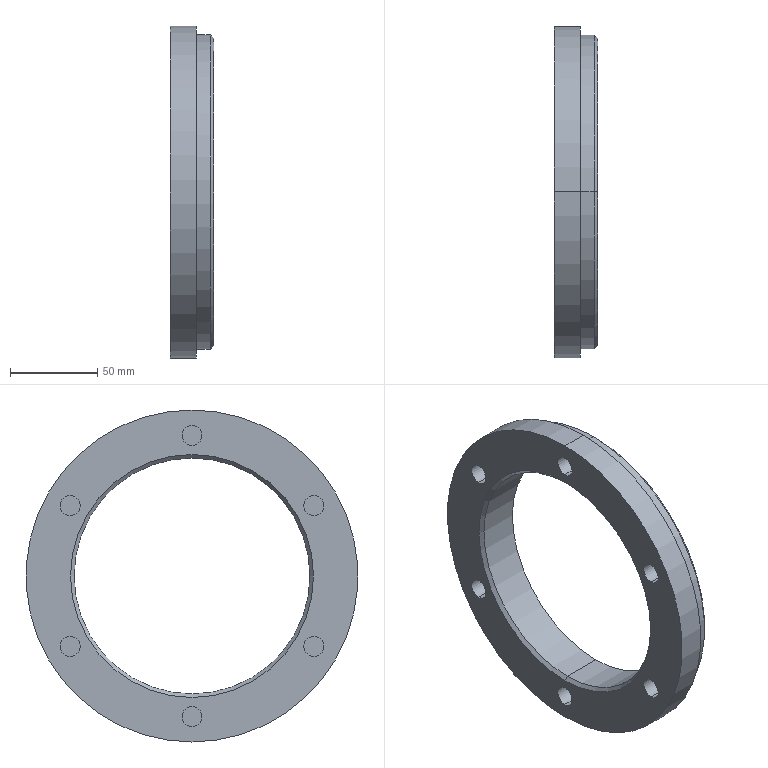Part | SolidWorks | features ICE 2, Chamfer 1, Extrusion 1 | 1 solid | 31 faces | box 25 x 190 x 190 mm | volume 309030 mm3 | cylinder 18 | plane 9 | cone 4 | commonest cylinder face diameters 11.5 x12 135 x2 180 x2 190 x2
STEP:
#1=CARTESIAN_POINT('',(25.,0.,-88.));
#2=VERTEX_POINT('',#1);
#3=CARTESIAN_POINT('',(25.,0.,88.));
#4=VERTEX_POINT('',#3);
#5=CARTESIAN_POINT('',(25.,0.,0.));
#6=DIRECTION('',(1.,0.,0.));
#7=DIRECTION('',(0.,0.,-1.));
#8=AXIS2_PLACEMENT_3D('',#5,#6,#7);
#9=CIRCLE('',#8,88.);
#10=EDGE_CURVE('',#2,#4,#9,.T.);
#11=ORIENTED_EDGE('',*,*,#10,.F.);
#12=CARTESIAN_POINT('',(23.,0.,-90.));
#13=VERTEX_POINT('',#12);
#14=CARTESIAN_POINT('',(25.,0.,-88.));
#15=DIRECTION('',(-0.7071,0.,-0.7071));
#16=VECTOR('',#15,1000.);
#17=LINE('',#14,#16);
#18=EDGE_CURVE('',#2,#13,#17,.T.);
#19=ORIENTED_EDGE('',*,*,#18,.T.);
#20=CARTESIAN_POINT('',(23.,0.,90.));
#21=VERTEX_POINT('',#20);
#22=CARTESIAN_POINT('',(23.,0.,0.));
#23=DIRECTION('',(-1.,0.,0.));
#24=DIRECTION('',(0.,0.,-1.));
#25=AXIS2_PLACEMENT_3D('',#22,#23,#24);
#26=CIRCLE('',#25,90.);
#27=EDGE_CURVE('',#21,#13,#26,.T.);
#28=ORIENTED_EDGE('',*,*,#27,.F.);
#29=CARTESIAN_POINT('',(25.,0.,88.));
#30=DIRECTION('',(-0.7071,0.,0.7071));
#31=VECTOR('',#30,1000.);
#32=LINE('',#29,#31);
#33=EDGE_CURVE('',#4,#21,#32,.T.);
#34=ORIENTED_EDGE('',*,*,#33,.F.);
#35=EDGE_LOOP('',(#11,#19,#28,#34));
#36=FACE_OUTER_BOUND('',#35,.T.);
#37=CARTESIAN_POINT('',(25.,0.,0.));
#38=DIRECTION('',(-1.,0.,0.));
#39=DIRECTION('',(0.,0.,1.));
#40=AXIS2_PLACEMENT_3D('',#37,#38,#39);
#41=CONICAL_SURFACE('',#40,88.,0.7854);
#42=ADVANCED_FACE('',(#36),#41,.T.);
#43=CARTESIAN_POINT('',(2.,0.,-67.5));
#44=VERTEX_POINT('',#43);
#45=CARTESIAN_POINT('',(2.,0.,67.5));
#46=VERTEX_POINT('',#45);
#47=CARTESIAN_POINT('',(2.,0.,0.));
#48=DIRECTION('',(-1.,0.,0.));
#49=DIRECTION('',(0.,0.,-1.));
#50=AXIS2_PLACEMENT_3D('',#47,#48,#49);
#51=CIRCLE('',#50,67.5);
#52=EDGE_CURVE('',#44,#46,#51,.T.);
#53=ORIENTED_EDGE('',*,*,#52,.F.);
#54=CARTESIAN_POINT('',(0.,0.,-69.5));
#55=VERTEX_POINT('',#54);
#56=CARTESIAN_POINT('',(0.,0.,-69.5));
#57=DIRECTION('',(-0.7071,0.,-0.7071));
#58=VECTOR('',#57,1000.);
#59=LINE('',#56,#58);
#60=EDGE_CURVE('',#44,#55,#59,.T.);
#61=ORIENTED_EDGE('',*,*,#60,.T.);
#62=CARTESIAN_POINT('',(0.,0.,69.5));
#63=VERTEX_POINT('',#62);
#64=CARTESIAN_POINT('',(0.,0.,0.));
#65=DIRECTION('',(1.,0.,0.));
#66=DIRECTION('',(0.,0.,-1.));
#67=AXIS2_PLACEMENT_3D('',#64,#65,#66);
#68=CIRCLE('',#67,69.5);
#69=EDGE_CURVE('',#63,#55,#68,.T.);
#70=ORIENTED_EDGE('',*,*,#69,.F.);
#71=CARTESIAN_POINT('',(0.,0.,69.5));
#72=DIRECTION('',(-0.7071,0.,0.7071));
#73=VECTOR('',#72,1000.);
#74=LINE('',#71,#73);
#75=EDGE_CURVE('',#46,#63,#74,.T.);
#76=ORIENTED_EDGE('',*,*,#75,.F.);
#77=EDGE_LOOP('',(#53,#61,#70,#76));
#78=FACE_OUTER_BOUND('',#77,.T.);
#79=CARTESIAN_POINT('',(0.,0.,0.));
#80=DIRECTION('',(-1.,0.,0.));
#81=DIRECTION('',(0.,0.,1.));
#82=AXIS2_PLACEMENT_3D('',#79,#80,#81);
#83=CONICAL_SURFACE('',#82,69.5,0.7854);
#84=ADVANCED_FACE('',(#78),#83,.F.);
#85=CARTESIAN_POINT('',(17.5,69.715,34.5));
#86=VERTEX_POINT('',#85);
#87=CARTESIAN_POINT('',(17.5,69.715,46.));
#88=VERTEX_POINT('',#87);
#89=CARTESIAN_POINT('',(17.5,69.715,40.25));
#90=DIRECTION('',(-1.,0.,0.));
#91=DIRECTION('',(0.,0.,1.));
#92=AXIS2_PLACEMENT_3D('',#89,#90,#91);
#93=CIRCLE('',#92,5.75);
#94=EDGE_CURVE('',#86,#88,#93,.T.);
#95=ORIENTED_EDGE('',*,*,#94,.F.);
#96=CARTESIAN_POINT('',(0.,69.715,34.5));
#97=VERTEX_POINT('',#96);
#98=CARTESIAN_POINT('',(17.5,69.715,34.5));
#99=DIRECTION('',(-1.,0.,0.));
#100=VECTOR('',#99,1000.);
#101=LINE('',#98,#100);
#102=EDGE_CURVE('',#86,#97,#101,.T.);
#103=ORIENTED_EDGE('',*,*,#102,.T.);
#104=CARTESIAN_POINT('',(0.,69.715,46.));
#105=VERTEX_POINT('',#104);
#106=CARTESIAN_POINT('',(0.,69.715,40.25));
#107=DIRECTION('',(-1.,0.,0.));
#108=DIRECTION('',(0.,0.,1.));
#109=AXIS2_PLACEMENT_3D('',#106,#107,#108);
#110=CIRCLE('',#109,5.75);
#111=EDGE_CURVE('',#97,#105,#110,.T.);
#112=ORIENTED_EDGE('',*,*,#111,.T.);
#113=CARTESIAN_POINT('',(17.5,69.715,46.));
#114=DIRECTION('',(-1.,0.,0.));
#115=VECTOR('',#114,1000.);
#116=LINE('',#113,#115);
#117=EDGE_CURVE('',#88,#105,#116,.T.);
#118=ORIENTED_EDGE('',*,*,#117,.F.);
#119=EDGE_LOOP('',(#95,#103,#112,#118));
#120=FACE_OUTER_BOUND('',#119,.T.);
#121=CARTESIAN_POINT('',(17.5,69.715,40.25));
#122=DIRECTION('',(-1.,0.,0.));
#123=DIRECTION('',(0.,0.,1.));
#124=AXIS2_PLACEMENT_3D('',#121,#122,#123);
#125=CYLINDRICAL_SURFACE('',#124,5.75);
#126=ADVANCED_FACE('',(#120),#125,.F.);
#127=CARTESIAN_POINT('',(17.5,69.715,-46.));
#128=VERTEX_POINT('',#127);
#129=CARTESIAN_POINT('',(17.5,69.715,-34.5));
#130=VERTEX_POINT('',#129);
#131=CARTESIAN_POINT('',(17.5,69.715,-40.25));
#132=DIRECTION('',(-1.,0.,0.));
#133=DIRECTION('',(0.,0.,1.));
#134=AXIS2_PLACEMENT_3D('',#131,#132,#133);
#135=CIRCLE('',#134,5.75);
#136=EDGE_CURVE('',#128,#130,#135,.T.);
#137=ORIENTED_EDGE('',*,*,#136,.F.);
#138=CARTESIAN_POINT('',(0.,69.715,-46.));
#139=VERTEX_POINT('',#138);
#140=CARTESIAN_POINT('',(17.5,69.715,-46.));
#141=DIRECTION('',(-1.,0.,0.));
#142=VECTOR('',#141,1000.);
#143=LINE('',#140,#142);
#144=EDGE_CURVE('',#128,#139,#143,.T.);
#145=ORIENTED_EDGE('',*,*,#144,.T.);
#146=CARTESIAN_POINT('',(0.,69.715,-34.5));
#147=VERTEX_POINT('',#146);
#148=CARTESIAN_POINT('',(0.,69.715,-40.25));
#149=DIRECTION('',(-1.,0.,0.));
#150=DIRECTION('',(0.,0.,1.));
#151=AXIS2_PLACEMENT_3D('',#148,#149,#150);
#152=CIRCLE('',#151,5.75);
#153=EDGE_CURVE('',#139,#147,#152,.T.);
#154=ORIENTED_EDGE('',*,*,#153,.T.);
#155=CARTESIAN_POINT('',(17.5,69.715,-34.5));
#156=DIRECTION('',(-1.,0.,0.));
#157=VECTOR('',#156,1000.);
#158=LINE('',#155,#157);
#159=EDGE_CURVE('',#130,#147,#158,.T.);
#160=ORIENTED_EDGE('',*,*,#159,.F.);
#161=EDGE_LOOP('',(#137,#145,#154,#160));
#162=FACE_OUTER_BOUND('',#161,.T.);
#163=CARTESIAN_POINT('',(17.5,69.715,-40.25));
#164=DIRECTION('',(-1.,0.,0.));
#165=DIRECTION('',(0.,0.,1.));
#166=AXIS2_PLACEMENT_3D('',#163,#164,#165);
#167=CYLINDRICAL_SURFACE('',#166,5.75);
#168=ADVANCED_FACE('',(#162),#167,.F.);
#169=CARTESIAN_POINT('',(17.5,0.,-86.25));
#170=VERTEX_POINT('',#169);
#171=CARTESIAN_POINT('',(17.5,0.,-74.75));
#172=VERTEX_POINT('',#171);
#173=CARTESIAN_POINT('',(17.5,0.,-80.5));
#174=DIRECTION('',(-1.,0.,0.));
#175=DIRECTION('',(0.,0.,1.));
#176=AXIS2_PLACEMENT_3D('',#173,#174,#175);
#177=CIRCLE('',#176,5.75);
#178=EDGE_CURVE('',#170,#172,#177,.T.);
#179=ORIENTED_EDGE('',*,*,#178,.F.);
#180=CARTESIAN_POINT('',(0.,0.,-86.25));
#181=VERTEX_POINT('',#180);
#182=CARTESIAN_POINT('',(17.5,0.,-86.25));
#183=DIRECTION('',(-1.,0.,0.));
#184=VECTOR('',#183,1000.);
#185=LINE('',#182,#184);
#186=EDGE_CURVE('',#170,#181,#185,.T.);
#187=ORIENTED_EDGE('',*,*,#186,.T.);
#188=CARTESIAN_POINT('',(0.,0.,-74.75));
#189=VERTEX_POINT('',#188);
#190=CARTESIAN_POINT('',(0.,0.,-80.5));
#191=DIRECTION('',(-1.,0.,0.));
#192=DIRECTION('',(0.,0.,1.));
#193=AXIS2_PLACEMENT_3D('',#190,#191,#192);
#194=CIRCLE('',#193,5.75);
#195=EDGE_CURVE('',#181,#189,#194,.T.);
#196=ORIENTED_EDGE('',*,*,#195,.T.);
#197=CARTESIAN_POINT('',(17.5,0.,-74.75));
#198=DIRECTION('',(-1.,0.,0.));
#199=VECTOR('',#198,1000.);
#200=LINE('',#197,#199);
#201=EDGE_CURVE('',#172,#189,#200,.T.);
#202=ORIENTED_EDGE('',*,*,#201,.F.);
#203=EDGE_LOOP('',(#179,#187,#196,#202));
#204=FACE_OUTER_BOUND('',#203,.T.);
#205=CARTESIAN_POINT('',(17.5,0.,-80.5));
#206=DIRECTION('',(-1.,0.,0.));
#207=DIRECTION('',(0.,0.,1.));
#208=AXIS2_PLACEMENT_3D('',#205,#206,#207);
#209=CYLINDRICAL_SURFACE('',#208,5.75);
#210=ADVANCED_FACE('',(#204),#209,.F.);
#211=CARTESIAN_POINT('',(17.5,-69.715,-46.));
#212=VERTEX_POINT('',#211);
#213=CARTESIAN_POINT('',(17.5,-69.715,-34.5));
#214=VERTEX_POINT('',#213);
#215=CARTESIAN_POINT('',(17.5,-69.715,-40.25));
#216=DIRECTION('',(-1.,0.,0.));
#217=DIRECTION('',(0.,0.,1.));
#218=AXIS2_PLACEMENT_3D('',#215,#216,#217);
#219=CIRCLE('',#218,5.75);
#220=EDGE_CURVE('',#212,#214,#219,.T.);
#221=ORIENTED_EDGE('',*,*,#220,.F.);
#222=CARTESIAN_POINT('',(0.,-69.715,-46.));
#223=VERTEX_POINT('',#222);
#224=CARTESIAN_POINT('',(17.5,-69.715,-46.));
#225=DIRECTION('',(-1.,0.,0.));
#226=VECTOR('',#225,1000.);
#227=LINE('',#224,#226);
#228=EDGE_CURVE('',#212,#223,#227,.T.);
#229=ORIENTED_EDGE('',*,*,#228,.T.);
#230=CARTESIAN_POINT('',(0.,-69.715,-34.5));
#231=VERTEX_POINT('',#230);
#232=CARTESIAN_POINT('',(0.,-69.715,-40.25));
#233=DIRECTION('',(-1.,0.,0.));
#234=DIRECTION('',(0.,0.,1.));
#235=AXIS2_PLACEMENT_3D('',#232,#233,#234);
#236=CIRCLE('',#235,5.75);
#237=EDGE_CURVE('',#223,#231,#236,.T.);
#238=ORIENTED_EDGE('',*,*,#237,.T.);
#239=CARTESIAN_POINT('',(17.5,-69.715,-34.5));
#240=DIRECTION('',(-1.,0.,0.));
#241=VECTOR('',#240,1000.);
#242=LINE('',#239,#241);
#243=EDGE_CURVE('',#214,#231,#242,.T.);
#244=ORIENTED_EDGE('',*,*,#243,.F.);
#245=EDGE_LOOP('',(#221,#229,#238,#244));
#246=FACE_OUTER_BOUND('',#245,.T.);
#247=CARTESIAN_POINT('',(17.5,-69.715,-40.25));
#248=DIRECTION('',(-1.,0.,0.));
#249=DIRECTION('',(0.,0.,1.));
#250=AXIS2_PLACEMENT_3D('',#247,#248,#249);
#251=CYLINDRICAL_SURFACE('',#250,5.75);
#252=ADVANCED_FACE('',(#246),#251,.F.);
#253=CARTESIAN_POINT('',(17.5,-69.715,34.5));
#254=VERTEX_POINT('',#253);
#255=CARTESIAN_POINT('',(17.5,-69.715,46.));
#256=VERTEX_POINT('',#255);
#257=CARTESIAN_POINT('',(17.5,-69.715,40.25));
#258=DIRECTION('',(-1.,0.,0.));
#259=DIRECTION('',(0.,0.,1.));
#260=AXIS2_PLACEMENT_3D('',#257,#258,#259);
#261=CIRCLE('',#260,5.75);
#262=EDGE_CURVE('',#254,#256,#261,.T.);
#263=ORIENTED_EDGE('',*,*,#262,.F.);
#264=CARTESIAN_POINT('',(0.,-69.715,34.5));
#265=VERTEX_POINT('',#264);
#266=CARTESIAN_POINT('',(17.5,-69.715,34.5));
#267=DIRECTION('',(-1.,0.,0.));
#268=VECTOR('',#267,1000.);
#269=LINE('',#266,#268);
#270=EDGE_CURVE('',#254,#265,#269,.T.);
#271=ORIENTED_EDGE('',*,*,#270,.T.);
#272=CARTESIAN_POINT('',(0.,-69.715,46.));
#273=VERTEX_POINT('',#272);
#274=CARTESIAN_POINT('',(0.,-69.715,40.25));
#275=DIRECTION('',(-1.,0.,0.));
#276=DIRECTION('',(0.,0.,1.));
#277=AXIS2_PLACEMENT_3D('',#274,#275,#276);
#278=CIRCLE('',#277,5.75);
#279=EDGE_CURVE('',#265,#273,#278,.T.);
#280=ORIENTED_EDGE('',*,*,#279,.T.);
#281=CARTESIAN_POINT('',(17.5,-69.715,46.));
#282=DIRECTION('',(-1.,0.,0.));
#283=VECTOR('',#282,1000.);
#284=LINE('',#281,#283);
#285=EDGE_CURVE('',#256,#273,#284,.T.);
#286=ORIENTED_EDGE('',*,*,#285,.F.);
#287=EDGE_LOOP('',(#263,#271,#280,#286));
#288=FACE_OUTER_BOUND('',#287,.T.);
#289=CARTESIAN_POINT('',(17.5,-69.715,40.25));
#290=DIRECTION('',(-1.,0.,0.));
#291=DIRECTION('',(0.,0.,1.));
#292=AXIS2_PLACEMENT_3D('',#289,#290,#291);
#293=CYLINDRICAL_SURFACE('',#292,5.75);
#294=ADVANCED_FACE('',(#288),#293,.F.);
#295=CARTESIAN_POINT('',(17.5,0.,74.75));
#296=VERTEX_POINT('',#295);
#297=CARTESIAN_POINT('',(17.5,0.,86.25));
#298=VERTEX_POINT('',#297);
#299=CARTESIAN_POINT('',(17.5,0.,80.5));
#300=DIRECTION('',(-1.,0.,0.));
#301=DIRECTION('',(0.,0.,1.));
#302=AXIS2_PLACEMENT_3D('',#299,#300,#301);
#303=CIRCLE('',#302,5.75);
#304=EDGE_CURVE('',#296,#298,#303,.T.);
#305=ORIENTED_EDGE('',*,*,#304,.F.);
#306=CARTESIAN_POINT('',(0.,0.,74.75));
#307=VERTEX_POINT('',#306);
#308=CARTESIAN_POINT('',(17.5,0.,74.75));
#309=DIRECTION('',(-1.,0.,0.));
#310=VECTOR('',#309,1000.);
#311=LINE('',#308,#310);
#312=EDGE_CURVE('',#296,#307,#311,.T.);
#313=ORIENTED_EDGE('',*,*,#312,.T.);
#314=CARTESIAN_POINT('',(0.,0.,86.25));
#315=VERTEX_POINT('',#314);
#316=CARTESIAN_POINT('',(0.,0.,80.5));
#317=DIRECTION('',(-1.,0.,0.));
#318=DIRECTION('',(0.,0.,1.));
#319=AXIS2_PLACEMENT_3D('',#316,#317,#318);
#320=CIRCLE('',#319,5.75);
#321=EDGE_CURVE('',#307,#315,#320,.T.);
#322=ORIENTED_EDGE('',*,*,#321,.T.);
#323=CARTESIAN_POINT('',(17.5,0.,86.25));
#324=DIRECTION('',(-1.,0.,0.));
#325=VECTOR('',#324,1000.);
#326=LINE('',#323,#325);
#327=EDGE_CURVE('',#298,#315,#326,.T.);
#328=ORIENTED_EDGE('',*,*,#327,.F.);
#329=EDGE_LOOP('',(#305,#313,#322,#328));
#330=FACE_OUTER_BOUND('',#329,.T.);
#331=CARTESIAN_POINT('',(17.5,0.,80.5));
#332=DIRECTION('',(-1.,0.,0.));
#333=DIRECTION('',(0.,0.,1.));
#334=AXIS2_PLACEMENT_3D('',#331,#332,#333);
#335=CYLINDRICAL_SURFACE('',#334,5.75);
#336=ADVANCED_FACE('',(#330),#335,.F.);
#337=CARTESIAN_POINT('',(15.,0.,-90.));
#338=VERTEX_POINT('',#337);
#339=CARTESIAN_POINT('',(15.,0.,90.));
#340=VERTEX_POINT('',#339);
#341=CARTESIAN_POINT('',(15.,0.,0.));
#342=DIRECTION('',(1.,0.,0.));
#343=DIRECTION('',(0.,0.,-1.));
#344=AXIS2_PLACEMENT_3D('',#341,#342,#343);
#345=CIRCLE('',#344,90.);
#346=EDGE_CURVE('',#338,#340,#345,.T.);
#347=ORIENTED_EDGE('',*,*,#346,.T.);
#348=CARTESIAN_POINT('',(15.,0.,90.));
#349=DIRECTION('',(1.,0.,0.));
#350=VECTOR('',#349,1000.);
#351=LINE('',#348,#350);
#352=EDGE_CURVE('',#340,#21,#351,.T.);
#353=ORIENTED_EDGE('',*,*,#352,.T.);
#354=ORIENTED_EDGE('',*,*,#27,.T.);
#355=CARTESIAN_POINT('',(15.,0.,-90.));
#356=DIRECTION('',(1.,0.,0.));
#357=VECTOR('',#356,1000.);
#358=LINE('',#355,#357);
#359=EDGE_CURVE('',#338,#13,#358,.T.);
#360=ORIENTED_EDGE('',*,*,#359,.F.);
#361=EDGE_LOOP('',(#347,#353,#354,#360));
#362=FACE_OUTER_BOUND('',#361,.T.);
#363=CARTESIAN_POINT('',(15.,0.,0.));
#364=DIRECTION('',(1.,0.,0.));
#365=DIRECTION('',(0.,0.,-1.));
#366=AXIS2_PLACEMENT_3D('',#363,#364,#365);
#367=CYLINDRICAL_SURFACE('',#366,90.);
#368=ADVANCED_FACE('',(#362),#367,.T.);
#369=CARTESIAN_POINT('',(25.,0.,67.5));
#370=VERTEX_POINT('',#369);
#371=CARTESIAN_POINT('',(25.,0.,-67.5));
#372=VERTEX_POINT('',#371);
#373=CARTESIAN_POINT('',(25.,0.,0.));
#374=DIRECTION('',(1.,0.,0.));
#375=DIRECTION('',(0.,0.,-1.));
#376=AXIS2_PLACEMENT_3D('',#373,#374,#375);
#377=CIRCLE('',#376,67.5);
#378=EDGE_CURVE('',#370,#372,#377,.T.);
#379=ORIENTED_EDGE('',*,*,#378,.T.);
#380=CARTESIAN_POINT('',(25.,0.,-67.5));
#381=DIRECTION('',(-1.,0.,0.));
#382=VECTOR('',#381,1000.);
#383=LINE('',#380,#382);
#384=EDGE_CURVE('',#372,#44,#383,.T.);
#385=ORIENTED_EDGE('',*,*,#384,.T.);
#386=ORIENTED_EDGE('',*,*,#52,.T.);
#387=CARTESIAN_POINT('',(25.,0.,67.5));
#388=DIRECTION('',(-1.,0.,0.));
#389=VECTOR('',#388,1000.);
#390=LINE('',#387,#389);
#391=EDGE_CURVE('',#370,#46,#390,.T.);
#392=ORIENTED_EDGE('',*,*,#391,.F.);
#393=EDGE_LOOP('',(#379,#385,#386,#392));
#394=FACE_OUTER_BOUND('',#393,.T.);
#395=CARTESIAN_POINT('',(25.,0.,0.));
#396=DIRECTION('',(-1.,0.,0.));
#397=DIRECTION('',(0.,0.,1.));
#398=AXIS2_PLACEMENT_3D('',#395,#396,#397);
#399=CYLINDRICAL_SURFACE('',#398,67.5);
#400=ADVANCED_FACE('',(#394),#399,.F.);
#401=CARTESIAN_POINT('',(15.,0.,-95.));
#402=VERTEX_POINT('',#401);
#403=CARTESIAN_POINT('',(15.,0.,95.));
#404=VERTEX_POINT('',#403);
#405=CARTESIAN_POINT('',(15.,0.,0.));
#406=DIRECTION('',(1.,0.,0.));
#407=DIRECTION('',(0.,0.,-1.));
#408=AXIS2_PLACEMENT_3D('',#405,#406,#407);
#409=CIRCLE('',#408,95.);
#410=EDGE_CURVE('',#402,#404,#409,.T.);
#411=ORIENTED_EDGE('',*,*,#410,.F.);
#412=CARTESIAN_POINT('',(0.,0.,-95.));
#413=VERTEX_POINT('',#412);
#414=CARTESIAN_POINT('',(25.,0.,-95.));
#415=DIRECTION('',(-1.,0.,0.));
#416=VECTOR('',#415,1000.);
#417=LINE('',#414,#416);
#418=EDGE_CURVE('',#402,#413,#417,.T.);
#419=ORIENTED_EDGE('',*,*,#418,.T.);
#420=CARTESIAN_POINT('',(0.,0.,95.));
#421=VERTEX_POINT('',#420);
#422=CARTESIAN_POINT('',(0.,0.,0.));
#423=DIRECTION('',(1.,0.,0.));
#424=DIRECTION('',(0.,0.,-1.));
#425=AXIS2_PLACEMENT_3D('',#422,#423,#424);
#426=CIRCLE('',#425,95.);
#427=EDGE_CURVE('',#413,#421,#426,.T.);
#428=ORIENTED_EDGE('',*,*,#427,.T.);
#429=CARTESIAN_POINT('',(25.,0.,95.));
#430=DIRECTION('',(-1.,0.,0.));
#431=VECTOR('',#430,1000.);
#432=LINE('',#429,#431);
#433=EDGE_CURVE('',#404,#421,#432,.T.);
#434=ORIENTED_EDGE('',*,*,#433,.F.);
#435=EDGE_LOOP('',(#411,#419,#428,#434));
#436=FACE_OUTER_BOUND('',#435,.T.);
#437=CARTESIAN_POINT('',(25.,0.,0.));
#438=DIRECTION('',(-1.,0.,0.));
#439=DIRECTION('',(0.,0.,1.));
#440=AXIS2_PLACEMENT_3D('',#437,#438,#439);
#441=CYLINDRICAL_SURFACE('',#440,95.);
#442=ADVANCED_FACE('',(#436),#441,.T.);
#443=CARTESIAN_POINT('',(25.,0.,0.));
#444=DIRECTION('',(1.,0.,0.));
#445=DIRECTION('',(0.,0.,-1.));
#446=AXIS2_PLACEMENT_3D('',#443,#444,#445);
#447=CIRCLE('',#446,88.);
#448=EDGE_CURVE('',#4,#2,#447,.T.);
#449=ORIENTED_EDGE('',*,*,#448,.T.);
#450=ORIENTED_EDGE('',*,*,#10,.T.);
#451=EDGE_LOOP('',(#449,#450));
#452=FACE_OUTER_BOUND('',#451,.T.);
#453=ORIENTED_EDGE('',*,*,#378,.F.);
#454=CARTESIAN_POINT('',(25.,0.,0.));
#455=DIRECTION('',(1.,0.,0.));
#456=DIRECTION('',(0.,0.,-1.));
#457=AXIS2_PLACEMENT_3D('',#454,#455,#456);
#458=CIRCLE('',#457,67.5);
#459=EDGE_CURVE('',#372,#370,#458,.T.);
#460=ORIENTED_EDGE('',*,*,#459,.F.);
#461=EDGE_LOOP('',(#453,#460));
#462=FACE_BOUND('',#461,.T.);
#463=CARTESIAN_POINT('',(25.,0.,0.));
#464=DIRECTION('',(1.,0.,0.));
#465=DIRECTION('',(0.,0.,-1.));
#466=AXIS2_PLACEMENT_3D('',#463,#464,#465);
#467=PLANE('',#466);
#468=ADVANCED_FACE('',(#452,#462),#467,.T.);
#469=ORIENTED_EDGE('',*,*,#418,.F.);
#470=CARTESIAN_POINT('',(15.,0.,0.));
#471=DIRECTION('',(1.,0.,0.));
#472=DIRECTION('',(0.,0.,-1.));
#473=AXIS2_PLACEMENT_3D('',#470,#471,#472);
#474=CIRCLE('',#473,95.);
#475=EDGE_CURVE('',#404,#402,#474,.T.);
#476=ORIENTED_EDGE('',*,*,#475,.F.);
#477=ORIENTED_EDGE('',*,*,#433,.T.);
#478=CARTESIAN_POINT('',(0.,0.,0.));
#479=DIRECTION('',(1.,0.,0.));
#480=DIRECTION('',(0.,0.,-1.));
#481=AXIS2_PLACEMENT_3D('',#478,#479,#480);
#482=CIRCLE('',#481,95.);
#483=EDGE_CURVE('',#421,#413,#482,.T.);
#484=ORIENTED_EDGE('',*,*,#483,.T.);
#485=EDGE_LOOP('',(#469,#476,#477,#484));
#486=FACE_OUTER_BOUND('',#485,.T.);
#487=CARTESIAN_POINT('',(25.,0.,0.));
#488=DIRECTION('',(-1.,0.,0.));
#489=DIRECTION('',(0.,0.,1.));
#490=AXIS2_PLACEMENT_3D('',#487,#488,#489);
#491=CYLINDRICAL_SURFACE('',#490,95.);
#492=ADVANCED_FACE('',(#486),#491,.T.);
#493=ORIENTED_EDGE('',*,*,#69,.T.);
#494=CARTESIAN_POINT('',(0.,0.,0.));
#495=DIRECTION('',(1.,0.,0.));
#496=DIRECTION('',(0.,0.,-1.));
#497=AXIS2_PLACEMENT_3D('',#494,#495,#496);
#498=CIRCLE('',#497,69.5);
#499=EDGE_CURVE('',#55,#63,#498,.T.);
#500=ORIENTED_EDGE('',*,*,#499,.T.);
#501=EDGE_LOOP('',(#493,#500));
#502=FACE_BOUND('',#501,.T.);
#503=CARTESIAN_POINT('',(0.,69.715,40.25));
#504=DIRECTION('',(-1.,0.,0.));
#505=DIRECTION('',(0.,0.,1.));
#506=AXIS2_PLACEMENT_3D('',#503,#504,#505);
#507=CIRCLE('',#506,5.75);
#508=EDGE_CURVE('',#105,#97,#507,.T.);
#509=ORIENTED_EDGE('',*,*,#508,.F.);
#510=ORIENTED_EDGE('',*,*,#111,.F.);
#511=EDGE_LOOP('',(#509,#510));
#512=FACE_BOUND('',#511,.T.);
#513=CARTESIAN_POINT('',(0.,69.715,-40.25));
#514=DIRECTION('',(-1.,0.,0.));
#515=DIRECTION('',(0.,0.,1.));
#516=AXIS2_PLACEMENT_3D('',#513,#514,#515);
#517=CIRCLE('',#516,5.75);
#518=EDGE_CURVE('',#147,#139,#517,.T.);
#519=ORIENTED_EDGE('',*,*,#518,.F.);
#520=ORIENTED_EDGE('',*,*,#153,.F.);
#521=EDGE_LOOP('',(#519,#520));
#522=FACE_BOUND('',#521,.T.);
#523=CARTESIAN_POINT('',(0.,0.,-80.5));
#524=DIRECTION('',(-1.,0.,0.));
#525=DIRECTION('',(0.,0.,1.));
#526=AXIS2_PLACEMENT_3D('',#523,#524,#525);
#527=CIRCLE('',#526,5.75);
#528=EDGE_CURVE('',#189,#181,#527,.T.);
#529=ORIENTED_EDGE('',*,*,#528,.F.);
#530=ORIENTED_EDGE('',*,*,#195,.F.);
#531=EDGE_LOOP('',(#529,#530));
#532=FACE_BOUND('',#531,.T.);
#533=CARTESIAN_POINT('',(0.,-69.715,-40.25));
#534=DIRECTION('',(-1.,0.,0.));
#535=DIRECTION('',(0.,0.,1.));
#536=AXIS2_PLACEMENT_3D('',#533,#534,#535);
#537=CIRCLE('',#536,5.75);
#538=EDGE_CURVE('',#231,#223,#537,.T.);
#539=ORIENTED_EDGE('',*,*,#538,.F.);
#540=ORIENTED_EDGE('',*,*,#237,.F.);
#541=EDGE_LOOP('',(#539,#540));
#542=FACE_BOUND('',#541,.T.);
#543=CARTESIAN_POINT('',(0.,-69.715,40.25));
#544=DIRECTION('',(-1.,0.,0.));
#545=DIRECTION('',(0.,0.,1.));
#546=AXIS2_PLACEMENT_3D('',#543,#544,#545);
#547=CIRCLE('',#546,5.75);
#548=EDGE_CURVE('',#273,#265,#547,.T.);
#549=ORIENTED_EDGE('',*,*,#548,.F.);
#550=ORIENTED_EDGE('',*,*,#279,.F.);
#551=EDGE_LOOP('',(#549,#550));
#552=FACE_BOUND('',#551,.T.);
#553=CARTESIAN_POINT('',(0.,0.,80.5));
#554=DIRECTION('',(-1.,0.,0.));
#555=DIRECTION('',(0.,0.,1.));
#556=AXIS2_PLACEMENT_3D('',#553,#554,#555);
#557=CIRCLE('',#556,5.75);
#558=EDGE_CURVE('',#315,#307,#557,.T.);
#559=ORIENTED_EDGE('',*,*,#558,.F.);
#560=ORIENTED_EDGE('',*,*,#321,.F.);
#561=EDGE_LOOP('',(#559,#560));
#562=FACE_BOUND('',#561,.T.);
#563=ORIENTED_EDGE('',*,*,#483,.F.);
#564=ORIENTED_EDGE('',*,*,#427,.F.);
#565=EDGE_LOOP('',(#563,#564));
#566=FACE_OUTER_BOUND('',#565,.T.);
#567=CARTESIAN_POINT('',(0.,0.,0.));
#568=DIRECTION('',(1.,0.,0.));
#569=DIRECTION('',(0.,0.,-1.));
#570=AXIS2_PLACEMENT_3D('',#567,#568,#569);
#571=PLANE('',#570);
#572=ADVANCED_FACE('',(#502,#512,#522,#532,#542,#552,#562,#566),#571,.F.);
#573=ORIENTED_EDGE('',*,*,#384,.F.);
#574=ORIENTED_EDGE('',*,*,#459,.T.);
#575=ORIENTED_EDGE('',*,*,#391,.T.);
#576=CARTESIAN_POINT('',(2.,0.,0.));
#577=DIRECTION('',(-1.,0.,0.));
#578=DIRECTION('',(0.,0.,-1.));
#579=AXIS2_PLACEMENT_3D('',#576,#577,#578);
#580=CIRCLE('',#579,67.5);
#581=EDGE_CURVE('',#46,#44,#580,.T.);
#582=ORIENTED_EDGE('',*,*,#581,.T.);
#583=EDGE_LOOP('',(#573,#574,#575,#582));
#584=FACE_OUTER_BOUND('',#583,.T.);
#585=CARTESIAN_POINT('',(25.,0.,0.));
#586=DIRECTION('',(-1.,0.,0.));
#587=DIRECTION('',(0.,0.,1.));
#588=AXIS2_PLACEMENT_3D('',#585,#586,#587);
#589=CYLINDRICAL_SURFACE('',#588,67.5);
#590=ADVANCED_FACE('',(#584),#589,.F.);
#591=ORIENTED_EDGE('',*,*,#346,.F.);
#592=CARTESIAN_POINT('',(15.,0.,0.));
#593=DIRECTION('',(1.,0.,0.));
#594=DIRECTION('',(0.,0.,-1.));
#595=AXIS2_PLACEMENT_3D('',#592,#593,#594);
#596=CIRCLE('',#595,90.);
#597=EDGE_CURVE('',#340,#338,#596,.T.);
#598=ORIENTED_EDGE('',*,*,#597,.F.);
#599=EDGE_LOOP('',(#591,#598));
#600=FACE_BOUND('',#599,.T.);
#601=ORIENTED_EDGE('',*,*,#475,.T.);
#602=ORIENTED_EDGE('',*,*,#410,.T.);
#603=EDGE_LOOP('',(#601,#602));
#604=FACE_OUTER_BOUND('',#603,.T.);
#605=CARTESIAN_POINT('',(15.,0.,0.));
#606=DIRECTION('',(1.,0.,0.));
#607=DIRECTION('',(0.,0.,-1.));
#608=AXIS2_PLACEMENT_3D('',#605,#606,#607);
#609=PLANE('',#608);
#610=ADVANCED_FACE('',(#600,#604),#609,.T.);
#611=ORIENTED_EDGE('',*,*,#352,.F.);
#612=ORIENTED_EDGE('',*,*,#597,.T.);
#613=ORIENTED_EDGE('',*,*,#359,.T.);
#614=CARTESIAN_POINT('',(23.,0.,0.));
#615=DIRECTION('',(-1.,0.,0.));
#616=DIRECTION('',(0.,0.,-1.));
#617=AXIS2_PLACEMENT_3D('',#614,#615,#616);
#618=CIRCLE('',#617,90.);
#619=EDGE_CURVE('',#13,#21,#618,.T.);
#620=ORIENTED_EDGE('',*,*,#619,.T.);
#621=EDGE_LOOP('',(#611,#612,#613,#620));
#622=FACE_OUTER_BOUND('',#621,.T.);
#623=CARTESIAN_POINT('',(15.,0.,0.));
#624=DIRECTION('',(1.,0.,0.));
#625=DIRECTION('',(0.,0.,-1.));
#626=AXIS2_PLACEMENT_3D('',#623,#624,#625);
#627=CYLINDRICAL_SURFACE('',#626,90.);
#628=ADVANCED_FACE('',(#622),#627,.T.);
#629=ORIENTED_EDGE('',*,*,#312,.F.);
#630=CARTESIAN_POINT('',(17.5,0.,80.5));
#631=DIRECTION('',(-1.,0.,0.));
#632=DIRECTION('',(0.,0.,1.));
#633=AXIS2_PLACEMENT_3D('',#630,#631,#632);
#634=CIRCLE('',#633,5.75);
#635=EDGE_CURVE('',#298,#296,#634,.T.);
#636=ORIENTED_EDGE('',*,*,#635,.F.);
#637=ORIENTED_EDGE('',*,*,#327,.T.);
#638=ORIENTED_EDGE('',*,*,#558,.T.);
#639=EDGE_LOOP('',(#629,#636,#637,#638));
#640=FACE_OUTER_BOUND('',#639,.T.);
#641=CARTESIAN_POINT('',(17.5,0.,80.5));
#642=DIRECTION('',(-1.,0.,0.));
#643=DIRECTION('',(0.,0.,1.));
#644=AXIS2_PLACEMENT_3D('',#641,#642,#643);
#645=CYLINDRICAL_SURFACE('',#644,5.75);
#646=ADVANCED_FACE('',(#640),#645,.F.);
#647=ORIENTED_EDGE('',*,*,#635,.T.);
#648=ORIENTED_EDGE('',*,*,#304,.T.);
#649=EDGE_LOOP('',(#647,#648));
#650=FACE_OUTER_BOUND('',#649,.T.);
#651=CARTESIAN_POINT('',(17.5,0.,80.5));
#652=DIRECTION('',(-1.,0.,0.));
#653=DIRECTION('',(0.,0.,1.));
#654=AXIS2_PLACEMENT_3D('',#651,#652,#653);
#655=PLANE('',#654);
#656=ADVANCED_FACE('',(#650),#655,.T.);
#657=ORIENTED_EDGE('',*,*,#270,.F.);
#658=CARTESIAN_POINT('',(17.5,-69.715,40.25));
#659=DIRECTION('',(-1.,0.,0.));
#660=DIRECTION('',(0.,0.,1.));
#661=AXIS2_PLACEMENT_3D('',#658,#659,#660);
#662=CIRCLE('',#661,5.75);
#663=EDGE_CURVE('',#256,#254,#662,.T.);
#664=ORIENTED_EDGE('',*,*,#663,.F.);
#665=ORIENTED_EDGE('',*,*,#285,.T.);
#666=ORIENTED_EDGE('',*,*,#548,.T.);
#667=EDGE_LOOP('',(#657,#664,#665,#666));
#668=FACE_OUTER_BOUND('',#667,.T.);
#669=CARTESIAN_POINT('',(17.5,-69.715,40.25));
#670=DIRECTION('',(-1.,0.,0.));
#671=DIRECTION('',(0.,0.,1.));
#672=AXIS2_PLACEMENT_3D('',#669,#670,#671);
#673=CYLINDRICAL_SURFACE('',#672,5.75);
#674=ADVANCED_FACE('',(#668),#673,.F.);
#675=ORIENTED_EDGE('',*,*,#663,.T.);
#676=ORIENTED_EDGE('',*,*,#262,.T.);
#677=EDGE_LOOP('',(#675,#676));
#678=FACE_OUTER_BOUND('',#677,.T.);
#679=CARTESIAN_POINT('',(17.5,-69.715,40.25));
#680=DIRECTION('',(-1.,0.,0.));
#681=DIRECTION('',(0.,0.,1.));
#682=AXIS2_PLACEMENT_3D('',#679,#680,#681);
#683=PLANE('',#682);
#684=ADVANCED_FACE('',(#678),#683,.T.);
#685=ORIENTED_EDGE('',*,*,#228,.F.);
#686=CARTESIAN_POINT('',(17.5,-69.715,-40.25));
#687=DIRECTION('',(-1.,0.,0.));
#688=DIRECTION('',(0.,0.,1.));
#689=AXIS2_PLACEMENT_3D('',#686,#687,#688);
#690=CIRCLE('',#689,5.75);
#691=EDGE_CURVE('',#214,#212,#690,.T.);
#692=ORIENTED_EDGE('',*,*,#691,.F.);
#693=ORIENTED_EDGE('',*,*,#243,.T.);
#694=ORIENTED_EDGE('',*,*,#538,.T.);
#695=EDGE_LOOP('',(#685,#692,#693,#694));
#696=FACE_OUTER_BOUND('',#695,.T.);
#697=CARTESIAN_POINT('',(17.5,-69.715,-40.25));
#698=DIRECTION('',(-1.,0.,0.));
#699=DIRECTION('',(0.,0.,1.));
#700=AXIS2_PLACEMENT_3D('',#697,#698,#699);
#701=CYLINDRICAL_SURFACE('',#700,5.75);
#702=ADVANCED_FACE('',(#696),#701,.F.);
#703=ORIENTED_EDGE('',*,*,#691,.T.);
#704=ORIENTED_EDGE('',*,*,#220,.T.);
#705=EDGE_LOOP('',(#703,#704));
#706=FACE_OUTER_BOUND('',#705,.T.);
#707=CARTESIAN_POINT('',(17.5,-69.715,-40.25));
#708=DIRECTION('',(-1.,0.,0.));
#709=DIRECTION('',(0.,0.,1.));
#710=AXIS2_PLACEMENT_3D('',#707,#708,#709);
#711=PLANE('',#710);
#712=ADVANCED_FACE('',(#706),#711,.T.);
#713=ORIENTED_EDGE('',*,*,#186,.F.);
#714=CARTESIAN_POINT('',(17.5,0.,-80.5));
#715=DIRECTION('',(-1.,0.,0.));
#716=DIRECTION('',(0.,0.,1.));
#717=AXIS2_PLACEMENT_3D('',#714,#715,#716);
#718=CIRCLE('',#717,5.75);
#719=EDGE_CURVE('',#172,#170,#718,.T.);
#720=ORIENTED_EDGE('',*,*,#719,.F.);
#721=ORIENTED_EDGE('',*,*,#201,.T.);
#722=ORIENTED_EDGE('',*,*,#528,.T.);
#723=EDGE_LOOP('',(#713,#720,#721,#722));
#724=FACE_OUTER_BOUND('',#723,.T.);
#725=CARTESIAN_POINT('',(17.5,0.,-80.5));
#726=DIRECTION('',(-1.,0.,0.));
#727=DIRECTION('',(0.,0.,1.));
#728=AXIS2_PLACEMENT_3D('',#725,#726,#727);
#729=CYLINDRICAL_SURFACE('',#728,5.75);
#730=ADVANCED_FACE('',(#724),#729,.F.);
#731=ORIENTED_EDGE('',*,*,#719,.T.);
#732=ORIENTED_EDGE('',*,*,#178,.T.);
#733=EDGE_LOOP('',(#731,#732));
#734=FACE_OUTER_BOUND('',#733,.T.);
#735=CARTESIAN_POINT('',(17.5,0.,-80.5));
#736=DIRECTION('',(-1.,0.,0.));
#737=DIRECTION('',(0.,0.,1.));
#738=AXIS2_PLACEMENT_3D('',#735,#736,#737);
#739=PLANE('',#738);
#740=ADVANCED_FACE('',(#734),#739,.T.);
#741=ORIENTED_EDGE('',*,*,#144,.F.);
#742=CARTESIAN_POINT('',(17.5,69.715,-40.25));
#743=DIRECTION('',(-1.,0.,0.));
#744=DIRECTION('',(0.,0.,1.));
#745=AXIS2_PLACEMENT_3D('',#742,#743,#744);
#746=CIRCLE('',#745,5.75);
#747=EDGE_CURVE('',#130,#128,#746,.T.);
#748=ORIENTED_EDGE('',*,*,#747,.F.);
#749=ORIENTED_EDGE('',*,*,#159,.T.);
#750=ORIENTED_EDGE('',*,*,#518,.T.);
#751=EDGE_LOOP('',(#741,#748,#749,#750));
#752=FACE_OUTER_BOUND('',#751,.T.);
#753=CARTESIAN_POINT('',(17.5,69.715,-40.25));
#754=DIRECTION('',(-1.,0.,0.));
#755=DIRECTION('',(0.,0.,1.));
#756=AXIS2_PLACEMENT_3D('',#753,#754,#755);
#757=CYLINDRICAL_SURFACE('',#756,5.75);
#758=ADVANCED_FACE('',(#752),#757,.F.);
#759=ORIENTED_EDGE('',*,*,#747,.T.);
#760=ORIENTED_EDGE('',*,*,#136,.T.);
#761=EDGE_LOOP('',(#759,#760));
#762=FACE_OUTER_BOUND('',#761,.T.);
#763=CARTESIAN_POINT('',(17.5,69.715,-40.25));
#764=DIRECTION('',(-1.,0.,0.));
#765=DIRECTION('',(0.,0.,1.));
#766=AXIS2_PLACEMENT_3D('',#763,#764,#765);
#767=PLANE('',#766);
#768=ADVANCED_FACE('',(#762),#767,.T.);
#769=ORIENTED_EDGE('',*,*,#102,.F.);
#770=CARTESIAN_POINT('',(17.5,69.715,40.25));
#771=DIRECTION('',(-1.,0.,0.));
#772=DIRECTION('',(0.,0.,1.));
#773=AXIS2_PLACEMENT_3D('',#770,#771,#772);
#774=CIRCLE('',#773,5.75);
#775=EDGE_CURVE('',#88,#86,#774,.T.);
#776=ORIENTED_EDGE('',*,*,#775,.F.);
#777=ORIENTED_EDGE('',*,*,#117,.T.);
#778=ORIENTED_EDGE('',*,*,#508,.T.);
#779=EDGE_LOOP('',(#769,#776,#777,#778));
#780=FACE_OUTER_BOUND('',#779,.T.);
#781=CARTESIAN_POINT('',(17.5,69.715,40.25));
#782=DIRECTION('',(-1.,0.,0.));
#783=DIRECTION('',(0.,0.,1.));
#784=AXIS2_PLACEMENT_3D('',#781,#782,#783);
#785=CYLINDRICAL_SURFACE('',#784,5.75);
#786=ADVANCED_FACE('',(#780),#785,.F.);
#787=ORIENTED_EDGE('',*,*,#775,.T.);
#788=ORIENTED_EDGE('',*,*,#94,.T.);
#789=EDGE_LOOP('',(#787,#788));
#790=FACE_OUTER_BOUND('',#789,.T.);
#791=CARTESIAN_POINT('',(17.5,69.715,40.25));
#792=DIRECTION('',(-1.,0.,0.));
#793=DIRECTION('',(0.,0.,1.));
#794=AXIS2_PLACEMENT_3D('',#791,#792,#793);
#795=PLANE('',#794);
#796=ADVANCED_FACE('',(#790),#795,.T.);
#797=ORIENTED_EDGE('',*,*,#60,.F.);
#798=ORIENTED_EDGE('',*,*,#581,.F.);
#799=ORIENTED_EDGE('',*,*,#75,.T.);
#800=ORIENTED_EDGE('',*,*,#499,.F.);
#801=EDGE_LOOP('',(#797,#798,#799,#800));
#802=FACE_OUTER_BOUND('',#801,.T.);
#803=CARTESIAN_POINT('',(0.,0.,0.));
#804=DIRECTION('',(-1.,0.,0.));
#805=DIRECTION('',(0.,0.,1.));
#806=AXIS2_PLACEMENT_3D('',#803,#804,#805);
#807=CONICAL_SURFACE('',#806,69.5,0.7854);
#808=ADVANCED_FACE('',(#802),#807,.F.);
#809=ORIENTED_EDGE('',*,*,#18,.F.);
#810=ORIENTED_EDGE('',*,*,#448,.F.);
#811=ORIENTED_EDGE('',*,*,#33,.T.);
#812=ORIENTED_EDGE('',*,*,#619,.F.);
#813=EDGE_LOOP('',(#809,#810,#811,#812));
#814=FACE_OUTER_BOUND('',#813,.T.);
#815=CARTESIAN_POINT('',(25.,0.,0.));
#816=DIRECTION('',(-1.,0.,0.));
#817=DIRECTION('',(0.,0.,1.));
#818=AXIS2_PLACEMENT_3D('',#815,#816,#817);
#819=CONICAL_SURFACE('',#818,88.,0.7854);
#820=ADVANCED_FACE('',(#814),#819,.T.);
#821=CLOSED_SHELL('',(#42,#84,#126,#168,#210,#252,#294,#336,#368,#400,#442,#468,#492,#572,#590,#610,#628,#646,#656,#674,#684,#702,#712,#730,#740,#758,#768,#786,#796,#808,#820));
#822=MANIFOLD_SOLID_BREP('',#821);
#823=CARTESIAN_POINT('',(0.,0.,0.));
#824=DIRECTION('',(0.,0.,1.));
#825=DIRECTION('',(1.,0.,0.));
#826=AXIS2_PLACEMENT_3D('',#823,#824,#825);
#827=(LENGTH_UNIT()NAMED_UNIT(*)SI_UNIT(.MILLI.,.METRE.));
#828=UNCERTAINTY_MEASURE_WITH_UNIT(LENGTH_MEASURE(0.00001),#827,'','');
#829=(NAMED_UNIT(*)PLANE_ANGLE_UNIT()SI_UNIT($,.RADIAN.));
#830=(NAMED_UNIT(*)SI_UNIT($,.STERADIAN.)SOLID_ANGLE_UNIT());
#831=(GEOMETRIC_REPRESENTATION_CONTEXT(3)GLOBAL_UNCERTAINTY_ASSIGNED_CONTEXT((#828))GLOBAL_UNIT_ASSIGNED_CONTEXT((#827,#829,#830))REPRESENTATION_CONTEXT('',''));
#832=ADVANCED_BREP_SHAPE_REPRESENTATION('',(#822,#826),#831);